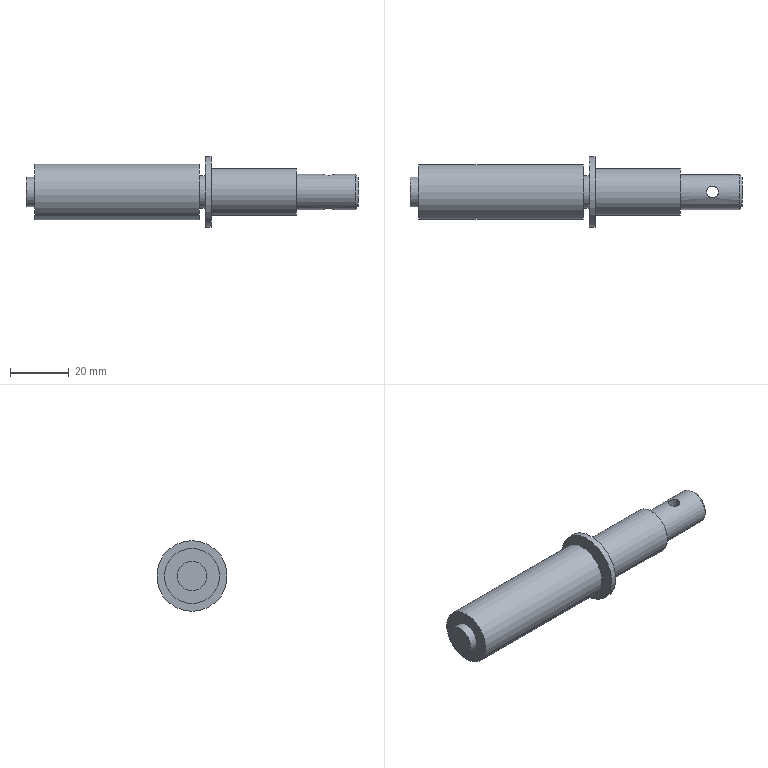Part | NX | features DATUM_CSYS 3, SKETCH 2, CHAMFER 1, EXTRUDE 1, SWP104 1 | 1 solid | 15 faces | box 113 x 24 x 24 mm | volume 24723 mm3 | cylinder 7 | plane 7 | cone 1 | commonest cylinder face diameters 4 x1 10 x1 11 x1 12 x1 15.821 x1 18.762 x1
STEP:
#1=CARTESIAN_POINT('',(-1.,0.,6.));
#2=VERTEX_POINT('',#1);
#3=CARTESIAN_POINT('',(-1.,0.,0.));
#4=DIRECTION('',(-1.,0.,0.));
#5=DIRECTION('',(0.,0.,1.));
#6=AXIS2_PLACEMENT_3D('',#3,#4,#5);
#7=CIRCLE('',#6,6.);
#8=EDGE_CURVE('',#2,#2,#7,.T.);
#9=ORIENTED_EDGE('',*,*,#8,.T.);
#10=EDGE_LOOP('',(#9));
#11=FACE_BOUND('',#10,.T.);
#12=CARTESIAN_POINT('',(-21.,0.,6.));
#13=VERTEX_POINT('',#12);
#14=CARTESIAN_POINT('',(-21.,0.,0.));
#15=DIRECTION('',(-1.,0.,0.));
#16=DIRECTION('',(0.,0.,1.));
#17=AXIS2_PLACEMENT_3D('',#14,#15,#16);
#18=CIRCLE('',#17,6.);
#19=EDGE_CURVE('',#13,#13,#18,.T.);
#20=ORIENTED_EDGE('',*,*,#19,.F.);
#21=EDGE_LOOP('',(#20));
#22=FACE_BOUND('',#21,.T.);
#23=CARTESIAN_POINT('',(-12.,0.,-6.));
#24=VERTEX_POINT('',#23);
#25=CARTESIAN_POINT('',(-11.566,-1.568,-5.833));
#26=CARTESIAN_POINT('',(-12.217,-0.00003474,-6.083));
#27=CARTESIAN_POINT('',(-11.566,1.568,-5.833));
#28=CARTESIAN_POINT('',(-10.003,2.216,-5.569));
#29=CARTESIAN_POINT('',(-8.432,1.567,-5.834));
#30=CARTESIAN_POINT('',(-7.784,0.001358,-6.083));
#31=CARTESIAN_POINT('',(-8.432,-1.567,-5.834));
#32=CARTESIAN_POINT('',(-10.,-2.216,-5.569));
#33=CARTESIAN_POINT('',(-11.566,-1.568,-5.833));
#34=CARTESIAN_POINT('',(-12.217,-0.00003474,-6.083));
#35=CARTESIAN_POINT('',(-11.566,1.568,-5.833));
#36=B_SPLINE_CURVE_WITH_KNOTS('',3,(#25,#26,#27,#28,#29,#30,#31,#32,#33,#34,#35),.UNSPECIFIED.,.T.,.F.,(1,1,1,1,1,1,1,1,1,1,1,1,1,1,1),(-0.004723,-0.003149,-0.001574,0.,0.001574,0.003149,0.004723,0.006298,0.007872,0.009446,0.01102,0.0126,0.01417,0.01574,0.01732),.UNSPECIFIED.);
#37=EDGE_CURVE('',#24,#24,#36,.T.);
#38=ORIENTED_EDGE('',*,*,#37,.F.);
#39=EDGE_LOOP('',(#38));
#40=FACE_BOUND('',#39,.T.);
#41=CARTESIAN_POINT('',(-8.,0.,6.));
#42=VERTEX_POINT('',#41);
#43=CARTESIAN_POINT('',(-8.434,-1.568,5.833));
#44=CARTESIAN_POINT('',(-7.783,-0.00003474,6.083));
#45=CARTESIAN_POINT('',(-8.434,1.568,5.833));
#46=CARTESIAN_POINT('',(-9.997,2.216,5.569));
#47=CARTESIAN_POINT('',(-11.568,1.567,5.834));
#48=CARTESIAN_POINT('',(-12.216,0.001358,6.083));
#49=CARTESIAN_POINT('',(-11.568,-1.567,5.834));
#50=CARTESIAN_POINT('',(-10.,-2.216,5.569));
#51=CARTESIAN_POINT('',(-8.434,-1.568,5.833));
#52=CARTESIAN_POINT('',(-7.783,-0.00003474,6.083));
#53=CARTESIAN_POINT('',(-8.434,1.568,5.833));
#54=B_SPLINE_CURVE_WITH_KNOTS('',3,(#43,#44,#45,#46,#47,#48,#49,#50,#51,#52,#53),.UNSPECIFIED.,.T.,.F.,(1,1,1,1,1,1,1,1,1,1,1,1,1,1,1),(-0.004723,-0.003149,-0.001574,0.,0.001574,0.003149,0.004723,0.006298,0.007872,0.009446,0.01102,0.0126,0.01417,0.01574,0.01732),.UNSPECIFIED.);
#55=EDGE_CURVE('',#42,#42,#54,.T.);
#56=ORIENTED_EDGE('',*,*,#55,.F.);
#57=EDGE_LOOP('',(#56));
#58=FACE_BOUND('',#57,.T.);
#59=CARTESIAN_POINT('',(0.,0.,0.));
#60=DIRECTION('',(-1.,0.,0.));
#61=DIRECTION('',(0.,0.,1.));
#62=AXIS2_PLACEMENT_3D('',#59,#60,#61);
#63=CYLINDRICAL_SURFACE('',#62,6.);
#64=ADVANCED_FACE('',(#11,#22,#40,#58),#63,.T.);
#65=CARTESIAN_POINT('',(-113.,0.,5.));
#66=VERTEX_POINT('',#65);
#67=CARTESIAN_POINT('',(-113.,0.,0.));
#68=DIRECTION('',(-1.,0.,0.));
#69=DIRECTION('',(0.,0.,1.));
#70=AXIS2_PLACEMENT_3D('',#67,#68,#69);
#71=CIRCLE('',#70,5.);
#72=EDGE_CURVE('',#66,#66,#71,.T.);
#73=ORIENTED_EDGE('',*,*,#72,.T.);
#74=EDGE_LOOP('',(#73));
#75=FACE_BOUND('',#74,.T.);
#76=CARTESIAN_POINT('',(-113.,5.,0.));
#77=DIRECTION('',(1.,0.,0.));
#78=DIRECTION('',(0.,0.,-1.));
#79=AXIS2_PLACEMENT_3D('',#76,#77,#78);
#80=PLANE('',#79);
#81=ADVANCED_FACE('',(#75),#80,.F.);
#82=CARTESIAN_POINT('',(0.,0.,5.));
#83=VERTEX_POINT('',#82);
#84=CARTESIAN_POINT('',(0.,0.,0.));
#85=DIRECTION('',(-1.,0.,0.));
#86=DIRECTION('',(0.,0.,1.));
#87=AXIS2_PLACEMENT_3D('',#84,#85,#86);
#88=CIRCLE('',#87,5.);
#89=EDGE_CURVE('',#83,#83,#88,.F.);
#90=ORIENTED_EDGE('',*,*,#89,.T.);
#91=EDGE_LOOP('',(#90));
#92=FACE_BOUND('',#91,.T.);
#93=CARTESIAN_POINT('',(0.,0.,0.));
#94=DIRECTION('',(-1.,0.,0.));
#95=DIRECTION('',(0.,0.,1.));
#96=AXIS2_PLACEMENT_3D('',#93,#94,#95);
#97=PLANE('',#96);
#98=ADVANCED_FACE('',(#92),#97,.F.);
#99=CARTESIAN_POINT('',(-21.,0.,7.911));
#100=VERTEX_POINT('',#99);
#101=CARTESIAN_POINT('',(-21.,0.,0.));
#102=DIRECTION('',(-1.,0.,0.));
#103=DIRECTION('',(0.,0.,1.));
#104=AXIS2_PLACEMENT_3D('',#101,#102,#103);
#105=CIRCLE('',#104,7.911);
#106=EDGE_CURVE('',#100,#100,#105,.T.);
#107=ORIENTED_EDGE('',*,*,#106,.F.);
#108=EDGE_LOOP('',(#107));
#109=FACE_BOUND('',#108,.T.);
#110=ORIENTED_EDGE('',*,*,#19,.T.);
#111=EDGE_LOOP('',(#110));
#112=FACE_BOUND('',#111,.T.);
#113=CARTESIAN_POINT('',(-21.,6.,0.));
#114=DIRECTION('',(-1.,0.,0.));
#115=DIRECTION('',(0.,0.,1.));
#116=AXIS2_PLACEMENT_3D('',#113,#114,#115);
#117=PLANE('',#116);
#118=ADVANCED_FACE('',(#109,#112),#117,.F.);
#119=CARTESIAN_POINT('',(-50.,0.,7.911));
#120=VERTEX_POINT('',#119);
#121=CARTESIAN_POINT('',(-50.,0.,0.));
#122=DIRECTION('',(-1.,0.,0.));
#123=DIRECTION('',(0.,0.,1.));
#124=AXIS2_PLACEMENT_3D('',#121,#122,#123);
#125=CIRCLE('',#124,7.911);
#126=EDGE_CURVE('',#120,#120,#125,.T.);
#127=ORIENTED_EDGE('',*,*,#126,.F.);
#128=EDGE_LOOP('',(#127));
#129=FACE_BOUND('',#128,.T.);
#130=ORIENTED_EDGE('',*,*,#106,.T.);
#131=EDGE_LOOP('',(#130));
#132=FACE_BOUND('',#131,.T.);
#133=CARTESIAN_POINT('',(0.,0.,0.));
#134=DIRECTION('',(-1.,0.,0.));
#135=DIRECTION('',(0.,0.,1.));
#136=AXIS2_PLACEMENT_3D('',#133,#134,#135);
#137=CYLINDRICAL_SURFACE('',#136,7.911);
#138=ADVANCED_FACE('',(#129,#132),#137,.T.);
#139=CARTESIAN_POINT('',(-50.,0.,12.));
#140=VERTEX_POINT('',#139);
#141=CARTESIAN_POINT('',(-50.,0.,0.));
#142=DIRECTION('',(-1.,0.,0.));
#143=DIRECTION('',(0.,0.,1.));
#144=AXIS2_PLACEMENT_3D('',#141,#142,#143);
#145=CIRCLE('',#144,12.);
#146=EDGE_CURVE('',#140,#140,#145,.T.);
#147=ORIENTED_EDGE('',*,*,#146,.F.);
#148=EDGE_LOOP('',(#147));
#149=FACE_BOUND('',#148,.T.);
#150=ORIENTED_EDGE('',*,*,#126,.T.);
#151=EDGE_LOOP('',(#150));
#152=FACE_BOUND('',#151,.T.);
#153=CARTESIAN_POINT('',(-50.,7.911,0.));
#154=DIRECTION('',(-1.,0.,0.));
#155=DIRECTION('',(0.,0.,1.));
#156=AXIS2_PLACEMENT_3D('',#153,#154,#155);
#157=PLANE('',#156);
#158=ADVANCED_FACE('',(#149,#152),#157,.F.);
#159=CARTESIAN_POINT('',(-52.,0.,12.));
#160=VERTEX_POINT('',#159);
#161=CARTESIAN_POINT('',(-52.,0.,0.));
#162=DIRECTION('',(-1.,0.,0.));
#163=DIRECTION('',(0.,0.,1.));
#164=AXIS2_PLACEMENT_3D('',#161,#162,#163);
#165=CIRCLE('',#164,12.);
#166=EDGE_CURVE('',#160,#160,#165,.T.);
#167=ORIENTED_EDGE('',*,*,#166,.F.);
#168=EDGE_LOOP('',(#167));
#169=FACE_BOUND('',#168,.T.);
#170=ORIENTED_EDGE('',*,*,#146,.T.);
#171=EDGE_LOOP('',(#170));
#172=FACE_BOUND('',#171,.T.);
#173=CARTESIAN_POINT('',(0.,0.,0.));
#174=DIRECTION('',(-1.,0.,0.));
#175=DIRECTION('',(0.,0.,1.));
#176=AXIS2_PLACEMENT_3D('',#173,#174,#175);
#177=CYLINDRICAL_SURFACE('',#176,12.);
#178=ADVANCED_FACE('',(#169,#172),#177,.T.);
#179=CARTESIAN_POINT('',(-52.,0.,5.5));
#180=VERTEX_POINT('',#179);
#181=CARTESIAN_POINT('',(-52.,0.,0.));
#182=DIRECTION('',(-1.,0.,0.));
#183=DIRECTION('',(0.,0.,1.));
#184=AXIS2_PLACEMENT_3D('',#181,#182,#183);
#185=CIRCLE('',#184,5.5);
#186=EDGE_CURVE('',#180,#180,#185,.T.);
#187=ORIENTED_EDGE('',*,*,#186,.F.);
#188=EDGE_LOOP('',(#187));
#189=FACE_BOUND('',#188,.T.);
#190=ORIENTED_EDGE('',*,*,#166,.T.);
#191=EDGE_LOOP('',(#190));
#192=FACE_BOUND('',#191,.T.);
#193=CARTESIAN_POINT('',(-52.,12.,0.));
#194=DIRECTION('',(1.,0.,0.));
#195=DIRECTION('',(0.,0.,-1.));
#196=AXIS2_PLACEMENT_3D('',#193,#194,#195);
#197=PLANE('',#196);
#198=ADVANCED_FACE('',(#189,#192),#197,.F.);
#199=CARTESIAN_POINT('',(-54.,0.,5.5));
#200=VERTEX_POINT('',#199);
#201=CARTESIAN_POINT('',(-54.,0.,0.));
#202=DIRECTION('',(-1.,0.,0.));
#203=DIRECTION('',(0.,0.,1.));
#204=AXIS2_PLACEMENT_3D('',#201,#202,#203);
#205=CIRCLE('',#204,5.5);
#206=EDGE_CURVE('',#200,#200,#205,.T.);
#207=ORIENTED_EDGE('',*,*,#206,.F.);
#208=EDGE_LOOP('',(#207));
#209=FACE_BOUND('',#208,.T.);
#210=ORIENTED_EDGE('',*,*,#186,.T.);
#211=EDGE_LOOP('',(#210));
#212=FACE_BOUND('',#211,.T.);
#213=CARTESIAN_POINT('',(0.,0.,0.));
#214=DIRECTION('',(-1.,0.,0.));
#215=DIRECTION('',(0.,0.,1.));
#216=AXIS2_PLACEMENT_3D('',#213,#214,#215);
#217=CYLINDRICAL_SURFACE('',#216,5.5);
#218=ADVANCED_FACE('',(#209,#212),#217,.T.);
#219=CARTESIAN_POINT('',(-54.,0.,9.381));
#220=VERTEX_POINT('',#219);
#221=CARTESIAN_POINT('',(-54.,0.,0.));
#222=DIRECTION('',(-1.,0.,0.));
#223=DIRECTION('',(0.,0.,1.));
#224=AXIS2_PLACEMENT_3D('',#221,#222,#223);
#225=CIRCLE('',#224,9.381);
#226=EDGE_CURVE('',#220,#220,#225,.T.);
#227=ORIENTED_EDGE('',*,*,#226,.F.);
#228=EDGE_LOOP('',(#227));
#229=FACE_BOUND('',#228,.T.);
#230=ORIENTED_EDGE('',*,*,#206,.T.);
#231=EDGE_LOOP('',(#230));
#232=FACE_BOUND('',#231,.T.);
#233=CARTESIAN_POINT('',(-54.,5.5,0.));
#234=DIRECTION('',(-1.,0.,0.));
#235=DIRECTION('',(0.,0.,1.));
#236=AXIS2_PLACEMENT_3D('',#233,#234,#235);
#237=PLANE('',#236);
#238=ADVANCED_FACE('',(#229,#232),#237,.F.);
#239=CARTESIAN_POINT('',(-110.,0.,9.381));
#240=VERTEX_POINT('',#239);
#241=CARTESIAN_POINT('',(-110.,0.,0.));
#242=DIRECTION('',(-1.,0.,0.));
#243=DIRECTION('',(0.,0.,1.));
#244=AXIS2_PLACEMENT_3D('',#241,#242,#243);
#245=CIRCLE('',#244,9.381);
#246=EDGE_CURVE('',#240,#240,#245,.T.);
#247=ORIENTED_EDGE('',*,*,#246,.F.);
#248=EDGE_LOOP('',(#247));
#249=FACE_BOUND('',#248,.T.);
#250=ORIENTED_EDGE('',*,*,#226,.T.);
#251=EDGE_LOOP('',(#250));
#252=FACE_BOUND('',#251,.T.);
#253=CARTESIAN_POINT('',(0.,0.,0.));
#254=DIRECTION('',(-1.,0.,0.));
#255=DIRECTION('',(0.,0.,1.));
#256=AXIS2_PLACEMENT_3D('',#253,#254,#255);
#257=CYLINDRICAL_SURFACE('',#256,9.381);
#258=ADVANCED_FACE('',(#249,#252),#257,.T.);
#259=CARTESIAN_POINT('',(-110.,0.,5.));
#260=VERTEX_POINT('',#259);
#261=CARTESIAN_POINT('',(-110.,0.,0.));
#262=DIRECTION('',(-1.,0.,0.));
#263=DIRECTION('',(0.,0.,1.));
#264=AXIS2_PLACEMENT_3D('',#261,#262,#263);
#265=CIRCLE('',#264,5.);
#266=EDGE_CURVE('',#260,#260,#265,.T.);
#267=ORIENTED_EDGE('',*,*,#266,.F.);
#268=EDGE_LOOP('',(#267));
#269=FACE_BOUND('',#268,.T.);
#270=ORIENTED_EDGE('',*,*,#246,.T.);
#271=EDGE_LOOP('',(#270));
#272=FACE_BOUND('',#271,.T.);
#273=CARTESIAN_POINT('',(-110.,9.381,0.));
#274=DIRECTION('',(1.,0.,0.));
#275=DIRECTION('',(0.,0.,-1.));
#276=AXIS2_PLACEMENT_3D('',#273,#274,#275);
#277=PLANE('',#276);
#278=ADVANCED_FACE('',(#269,#272),#277,.F.);
#279=ORIENTED_EDGE('',*,*,#72,.F.);
#280=EDGE_LOOP('',(#279));
#281=FACE_BOUND('',#280,.T.);
#282=ORIENTED_EDGE('',*,*,#266,.T.);
#283=EDGE_LOOP('',(#282));
#284=FACE_BOUND('',#283,.T.);
#285=CARTESIAN_POINT('',(0.,0.,0.));
#286=DIRECTION('',(-1.,0.,0.));
#287=DIRECTION('',(0.,0.,1.));
#288=AXIS2_PLACEMENT_3D('',#285,#286,#287);
#289=CYLINDRICAL_SURFACE('',#288,5.);
#290=ADVANCED_FACE('',(#281,#284),#289,.T.);
#291=ORIENTED_EDGE('',*,*,#89,.F.);
#292=EDGE_LOOP('',(#291));
#293=FACE_BOUND('',#292,.T.);
#294=ORIENTED_EDGE('',*,*,#8,.F.);
#295=EDGE_LOOP('',(#294));
#296=FACE_BOUND('',#295,.T.);
#297=CARTESIAN_POINT('',(-1.,0.,0.));
#298=DIRECTION('',(-1.,0.,0.));
#299=DIRECTION('',(0.,0.,1.));
#300=AXIS2_PLACEMENT_3D('',#297,#298,#299);
#301=CONICAL_SURFACE('',#300,6.,0.7854);
#302=ADVANCED_FACE('',(#293,#296),#301,.T.);
#303=ORIENTED_EDGE('',*,*,#37,.T.);
#304=EDGE_LOOP('',(#303));
#305=FACE_BOUND('',#304,.T.);
#306=ORIENTED_EDGE('',*,*,#55,.T.);
#307=EDGE_LOOP('',(#306));
#308=FACE_BOUND('',#307,.T.);
#309=CARTESIAN_POINT('',(-10.,0.,18.));
#310=DIRECTION('',(0.,0.,-1.));
#311=DIRECTION('',(-1.,0.,0.));
#312=AXIS2_PLACEMENT_3D('',#309,#310,#311);
#313=CYLINDRICAL_SURFACE('',#312,2.);
#314=ADVANCED_FACE('',(#305,#308),#313,.F.);
#315=CLOSED_SHELL('',(#64,#81,#98,#118,#138,#158,#178,#198,#218,#238,#258,#278,#290,#302,#314));
#316=MANIFOLD_SOLID_BREP('',#315);
#317=(LENGTH_UNIT()NAMED_UNIT(*)SI_UNIT(.MILLI.,.METRE.));
#318=UNCERTAINTY_MEASURE_WITH_UNIT(LENGTH_MEASURE(0.0508),#317,'','');
#319=(NAMED_UNIT(*)PLANE_ANGLE_UNIT()SI_UNIT($,.RADIAN.));
#320=(NAMED_UNIT(*)SI_UNIT($,.STERADIAN.)SOLID_ANGLE_UNIT());
#321=(GEOMETRIC_REPRESENTATION_CONTEXT(3)GLOBAL_UNCERTAINTY_ASSIGNED_CONTEXT((#318))GLOBAL_UNIT_ASSIGNED_CONTEXT((#317,#319,#320))REPRESENTATION_CONTEXT('',''));
#322=ADVANCED_BREP_SHAPE_REPRESENTATION('',(#316),#321);